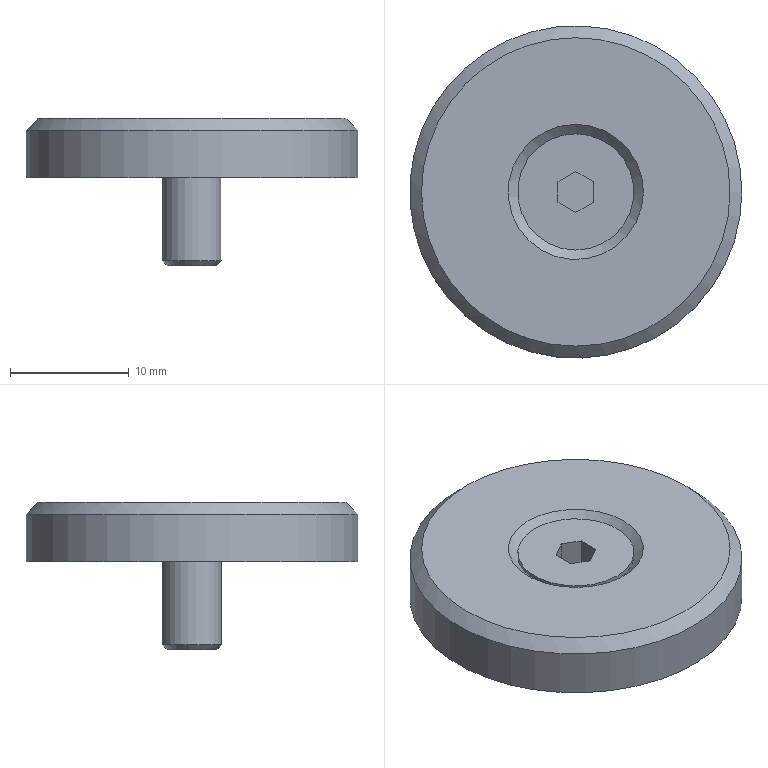Part | STEP file | STP | 2 solids | 19 faces | box 28 x 28 x 12.4 mm | volume 3112 mm3 | plane 11 | cylinder 4 | cone 4 | commonest cylinder face diameters 5 x1 5.5 x1 9.8 x1 28 x1
STEP:
#1=CARTESIAN_POINT('',(0.,0.,0.));
#2=DIRECTION('',(0.,0.,1.));
#3=DIRECTION('',(1.,0.,0.));
#4=AXIS2_PLACEMENT_3D('',#1,#2,#3);
#5=CARTESIAN_POINT('',(138.,294.1,-308.4));
#6=VERTEX_POINT('',#5);
#7=CARTESIAN_POINT('',(138.,289.9,-308.4));
#8=VERTEX_POINT('',#7);
#9=CARTESIAN_POINT('',(138.,292.,-308.4));
#10=DIRECTION('',(0.,0.,-1.));
#11=DIRECTION('',(0.,1.,0.));
#12=AXIS2_PLACEMENT_3D('',#9,#10,#11);
#13=CIRCLE('',#12,2.1);
#14=CARTESIAN_POINT('',(138.,292.,-308.4));
#15=DIRECTION('',(0.,0.,-1.));
#16=DIRECTION('',(0.,1.,0.));
#17=AXIS2_PLACEMENT_3D('',#14,#15,#16);
#18=PLANE('',#17);
#19=CARTESIAN_POINT('',(0.,0.));
#20=DIRECTION('',(1.,0.));
#21=AXIS2_PLACEMENT_2D('',#19,#20);
#22=CIRCLE('',#21,2.1);
#23=(GEOMETRIC_REPRESENTATION_CONTEXT(2)PARAMETRIC_REPRESENTATION_CONTEXT()REPRESENTATION_CONTEXT('',''));
#24=DEFINITIONAL_REPRESENTATION('',(#22),#23);
#25=PCURVE('',#18,#24);
#26=CARTESIAN_POINT('',(138.,292.,-308.));
#27=DIRECTION('',(0.,0.,1.));
#28=DIRECTION('',(0.,-1.,0.));
#29=AXIS2_PLACEMENT_3D('',#26,#27,#28);
#30=CONICAL_SURFACE('',#29,2.5,0.7854);
#31=CARTESIAN_POINT('',(3.142,-0.4));
#32=DIRECTION('',(-1.,0.));
#33=VECTOR('',#32,1.);
#34=LINE('',#31,#33);
#35=(GEOMETRIC_REPRESENTATION_CONTEXT(2)PARAMETRIC_REPRESENTATION_CONTEXT()REPRESENTATION_CONTEXT('',''));
#36=DEFINITIONAL_REPRESENTATION('',(#34),#35);
#37=PCURVE('',#30,#36);
#38=SURFACE_CURVE('',#13,(#25,#37),.PCURVE_S1.);
#39=EDGE_CURVE('',#6,#8,#38,.T.);
#40=ORIENTED_EDGE('',*,*,#39,.T.);
#41=CARTESIAN_POINT('',(138.,292.,-308.4));
#42=DIRECTION('',(0.,0.,-1.));
#43=DIRECTION('',(0.,1.,0.));
#44=AXIS2_PLACEMENT_3D('',#41,#42,#43);
#45=CIRCLE('',#44,2.1);
#46=CARTESIAN_POINT('',(0.,0.));
#47=DIRECTION('',(1.,0.));
#48=AXIS2_PLACEMENT_2D('',#46,#47);
#49=CIRCLE('',#48,2.1);
#50=(GEOMETRIC_REPRESENTATION_CONTEXT(2)PARAMETRIC_REPRESENTATION_CONTEXT()REPRESENTATION_CONTEXT('',''));
#51=DEFINITIONAL_REPRESENTATION('',(#49),#50);
#52=PCURVE('',#18,#51);
#53=CARTESIAN_POINT('',(9.425,-0.4));
#54=DIRECTION('',(-1.,0.));
#55=VECTOR('',#54,1.);
#56=LINE('',#53,#55);
#57=(GEOMETRIC_REPRESENTATION_CONTEXT(2)PARAMETRIC_REPRESENTATION_CONTEXT()REPRESENTATION_CONTEXT('',''));
#58=DEFINITIONAL_REPRESENTATION('',(#56),#57);
#59=PCURVE('',#30,#58);
#60=SURFACE_CURVE('',#45,(#52,#59),.PCURVE_S1.);
#61=EDGE_CURVE('',#8,#6,#60,.T.);
#62=ORIENTED_EDGE('',*,*,#61,.T.);
#63=EDGE_LOOP('',(#40,#62));
#64=FACE_BOUND('',#63,.T.);
#65=ADVANCED_FACE('',(#64),#18,.T.);
#66=CARTESIAN_POINT('',(138.,289.5,-308.));
#67=VERTEX_POINT('',#66);
#68=CARTESIAN_POINT('',(138.,292.,-308.));
#69=DIRECTION('',(0.,0.,1.));
#70=DIRECTION('',(0.,-1.,0.));
#71=AXIS2_PLACEMENT_3D('',#68,#69,#70);
#72=CIRCLE('',#71,2.5);
#73=CARTESIAN_POINT('',(138.,292.,-299.2));
#74=DIRECTION('',(0.,0.,-1.));
#75=DIRECTION('',(0.,1.,0.));
#76=AXIS2_PLACEMENT_3D('',#73,#74,#75);
#77=CYLINDRICAL_SURFACE('',#76,2.5);
#78=CARTESIAN_POINT('',(9.425,8.8));
#79=DIRECTION('',(-1.,0.));
#80=VECTOR('',#79,1.);
#81=LINE('',#78,#80);
#82=(GEOMETRIC_REPRESENTATION_CONTEXT(2)PARAMETRIC_REPRESENTATION_CONTEXT()REPRESENTATION_CONTEXT('',''));
#83=DEFINITIONAL_REPRESENTATION('',(#81),#82);
#84=PCURVE('',#77,#83);
#85=CARTESIAN_POINT('',(0.,0.));
#86=DIRECTION('',(1.,0.));
#87=VECTOR('',#86,1.);
#88=LINE('',#85,#87);
#89=(GEOMETRIC_REPRESENTATION_CONTEXT(2)PARAMETRIC_REPRESENTATION_CONTEXT()REPRESENTATION_CONTEXT('',''));
#90=DEFINITIONAL_REPRESENTATION('',(#88),#89);
#91=PCURVE('',#30,#90);
#92=SURFACE_CURVE('',#72,(#84,#91),.PCURVE_S1.);
#93=EDGE_CURVE('',#67,#67,#92,.T.);
#94=ORIENTED_EDGE('',*,*,#93,.T.);
#95=CARTESIAN_POINT('',(138.,289.5,-299.2));
#96=VERTEX_POINT('',#95);
#97=CARTESIAN_POINT('',(138.,289.5,-299.2));
#98=CARTESIAN_POINT('',(138.,289.5,-308.));
#99=B_SPLINE_CURVE_WITH_KNOTS('',1,(#97,#98),.UNSPECIFIED.,.F.,.F.,(2,2),(0.,8.8),.PIECEWISE_BEZIER_KNOTS.);
#100=CARTESIAN_POINT('',(3.142,0.));
#101=DIRECTION('',(0.,1.));
#102=VECTOR('',#101,1.);
#103=LINE('',#100,#102);
#104=(GEOMETRIC_REPRESENTATION_CONTEXT(2)PARAMETRIC_REPRESENTATION_CONTEXT()REPRESENTATION_CONTEXT('',''));
#105=DEFINITIONAL_REPRESENTATION('',(#103),#104);
#106=PCURVE('',#77,#105);
#107=CARTESIAN_POINT('',(9.425,0.));
#108=DIRECTION('',(0.,1.));
#109=VECTOR('',#108,1.);
#110=LINE('',#107,#109);
#111=(GEOMETRIC_REPRESENTATION_CONTEXT(2)PARAMETRIC_REPRESENTATION_CONTEXT()REPRESENTATION_CONTEXT('',''));
#112=DEFINITIONAL_REPRESENTATION('',(#110),#111);
#113=PCURVE('',#77,#112);
#114=SEAM_CURVE('',#99,(#106,#113),.PCURVE_S1.);
#115=EDGE_CURVE('',#96,#67,#114,.T.);
#116=ORIENTED_EDGE('',*,*,#115,.F.);
#117=CARTESIAN_POINT('',(138.,292.,-299.2));
#118=DIRECTION('',(0.,0.,1.));
#119=DIRECTION('',(0.,-1.,0.));
#120=AXIS2_PLACEMENT_3D('',#117,#118,#119);
#121=CIRCLE('',#120,2.5);
#122=CARTESIAN_POINT('',(9.425,0.));
#123=DIRECTION('',(-1.,0.));
#124=VECTOR('',#123,1.);
#125=LINE('',#122,#124);
#126=(GEOMETRIC_REPRESENTATION_CONTEXT(2)PARAMETRIC_REPRESENTATION_CONTEXT()REPRESENTATION_CONTEXT('',''));
#127=DEFINITIONAL_REPRESENTATION('',(#125),#126);
#128=PCURVE('',#77,#127);
#129=CARTESIAN_POINT('',(138.,292.,-299.2));
#130=DIRECTION('',(0.,0.,1.));
#131=DIRECTION('',(0.,1.,0.));
#132=AXIS2_PLACEMENT_3D('',#129,#130,#131);
#133=CONICAL_SURFACE('',#132,2.5,0.7854);
#134=CARTESIAN_POINT('',(3.142,0.));
#135=DIRECTION('',(1.,0.));
#136=VECTOR('',#135,1.);
#137=LINE('',#134,#136);
#138=(GEOMETRIC_REPRESENTATION_CONTEXT(2)PARAMETRIC_REPRESENTATION_CONTEXT()REPRESENTATION_CONTEXT('',''));
#139=DEFINITIONAL_REPRESENTATION('',(#137),#138);
#140=PCURVE('',#133,#139);
#141=SURFACE_CURVE('',#121,(#128,#140),.PCURVE_S1.);
#142=EDGE_CURVE('',#96,#96,#141,.T.);
#143=ORIENTED_EDGE('',*,*,#142,.F.);
#144=ORIENTED_EDGE('',*,*,#115,.T.);
#145=EDGE_LOOP('',(#94,#116,#143,#144));
#146=FACE_BOUND('',#145,.T.);
#147=ADVANCED_FACE('',(#146),#77,.T.);
#148=CARTESIAN_POINT('',(138.,287.1,-296.8));
#149=VERTEX_POINT('',#148);
#150=CARTESIAN_POINT('',(138.,292.,-296.8));
#151=DIRECTION('',(0.,0.,-1.));
#152=DIRECTION('',(0.,-1.,0.));
#153=AXIS2_PLACEMENT_3D('',#150,#151,#152);
#154=CIRCLE('',#153,4.9);
#155=CARTESIAN_POINT('',(9.425,2.4));
#156=DIRECTION('',(-1.,0.));
#157=VECTOR('',#156,1.);
#158=LINE('',#155,#157);
#159=(GEOMETRIC_REPRESENTATION_CONTEXT(2)PARAMETRIC_REPRESENTATION_CONTEXT()REPRESENTATION_CONTEXT('',''));
#160=DEFINITIONAL_REPRESENTATION('',(#158),#159);
#161=PCURVE('',#133,#160);
#162=CARTESIAN_POINT('',(138.,292.,-299.2));
#163=DIRECTION('',(0.,0.,1.));
#164=DIRECTION('',(0.,-1.,0.));
#165=AXIS2_PLACEMENT_3D('',#162,#163,#164);
#166=CYLINDRICAL_SURFACE('',#165,4.9);
#167=CARTESIAN_POINT('',(6.283,2.4));
#168=DIRECTION('',(-1.,0.));
#169=VECTOR('',#168,1.);
#170=LINE('',#167,#169);
#171=(GEOMETRIC_REPRESENTATION_CONTEXT(2)PARAMETRIC_REPRESENTATION_CONTEXT()REPRESENTATION_CONTEXT('',''));
#172=DEFINITIONAL_REPRESENTATION('',(#170),#171);
#173=PCURVE('',#166,#172);
#174=SURFACE_CURVE('',#154,(#161,#173),.PCURVE_S1.);
#175=EDGE_CURVE('',#149,#149,#174,.T.);
#176=ORIENTED_EDGE('',*,*,#175,.T.);
#177=CARTESIAN_POINT('',(138.,289.5,-299.2));
#178=CARTESIAN_POINT('',(138.,287.1,-296.8));
#179=B_SPLINE_CURVE_WITH_KNOTS('',1,(#177,#178),.UNSPECIFIED.,.F.,.F.,(2,2),(0.,3.394),.PIECEWISE_BEZIER_KNOTS.);
#180=CARTESIAN_POINT('',(3.142,0.));
#181=DIRECTION('',(0.,1.));
#182=VECTOR('',#181,1.);
#183=LINE('',#180,#182);
#184=(GEOMETRIC_REPRESENTATION_CONTEXT(2)PARAMETRIC_REPRESENTATION_CONTEXT()REPRESENTATION_CONTEXT('',''));
#185=DEFINITIONAL_REPRESENTATION('',(#183),#184);
#186=PCURVE('',#133,#185);
#187=CARTESIAN_POINT('',(9.425,0.));
#188=DIRECTION('',(0.,1.));
#189=VECTOR('',#188,1.);
#190=LINE('',#187,#189);
#191=(GEOMETRIC_REPRESENTATION_CONTEXT(2)PARAMETRIC_REPRESENTATION_CONTEXT()REPRESENTATION_CONTEXT('',''));
#192=DEFINITIONAL_REPRESENTATION('',(#190),#191);
#193=PCURVE('',#133,#192);
#194=SEAM_CURVE('',#179,(#186,#193),.PCURVE_S1.);
#195=EDGE_CURVE('',#96,#149,#194,.T.);
#196=ORIENTED_EDGE('',*,*,#195,.F.);
#197=ORIENTED_EDGE('',*,*,#142,.T.);
#198=ORIENTED_EDGE('',*,*,#195,.T.);
#199=EDGE_LOOP('',(#176,#196,#197,#198));
#200=FACE_BOUND('',#199,.T.);
#201=ADVANCED_FACE('',(#200),#133,.T.);
#202=CARTESIAN_POINT('',(138.,287.1,-296.4));
#203=VERTEX_POINT('',#202);
#204=CARTESIAN_POINT('',(138.,292.,-296.4));
#205=DIRECTION('',(0.,0.,1.));
#206=DIRECTION('',(0.,-1.,0.));
#207=AXIS2_PLACEMENT_3D('',#204,#205,#206);
#208=CIRCLE('',#207,4.9);
#209=CARTESIAN_POINT('',(0.,2.8));
#210=DIRECTION('',(1.,0.));
#211=VECTOR('',#210,1.);
#212=LINE('',#209,#211);
#213=(GEOMETRIC_REPRESENTATION_CONTEXT(2)PARAMETRIC_REPRESENTATION_CONTEXT()REPRESENTATION_CONTEXT('',''));
#214=DEFINITIONAL_REPRESENTATION('',(#212),#213);
#215=PCURVE('',#166,#214);
#216=CARTESIAN_POINT('',(138.,292.,-296.4));
#217=DIRECTION('',(0.,0.,1.));
#218=DIRECTION('',(0.,-1.,0.));
#219=AXIS2_PLACEMENT_3D('',#216,#217,#218);
#220=PLANE('',#219);
#221=CARTESIAN_POINT('',(0.,0.));
#222=DIRECTION('',(1.,0.));
#223=AXIS2_PLACEMENT_2D('',#221,#222);
#224=CIRCLE('',#223,4.9);
#225=(GEOMETRIC_REPRESENTATION_CONTEXT(2)PARAMETRIC_REPRESENTATION_CONTEXT()REPRESENTATION_CONTEXT('',''));
#226=DEFINITIONAL_REPRESENTATION('',(#224),#225);
#227=PCURVE('',#220,#226);
#228=SURFACE_CURVE('',#208,(#215,#227),.PCURVE_S1.);
#229=EDGE_CURVE('',#203,#203,#228,.T.);
#230=ORIENTED_EDGE('',*,*,#229,.F.);
#231=CARTESIAN_POINT('',(138.,287.1,-296.8));
#232=CARTESIAN_POINT('',(138.,287.1,-296.4));
#233=B_SPLINE_CURVE_WITH_KNOTS('',1,(#231,#232),.UNSPECIFIED.,.F.,.F.,(2,2),(2.4,2.8),.PIECEWISE_BEZIER_KNOTS.);
#234=CARTESIAN_POINT('',(0.,0.));
#235=DIRECTION('',(0.,1.));
#236=VECTOR('',#235,1.);
#237=LINE('',#234,#236);
#238=(GEOMETRIC_REPRESENTATION_CONTEXT(2)PARAMETRIC_REPRESENTATION_CONTEXT()REPRESENTATION_CONTEXT('',''));
#239=DEFINITIONAL_REPRESENTATION('',(#237),#238);
#240=PCURVE('',#166,#239);
#241=CARTESIAN_POINT('',(6.283,0.));
#242=DIRECTION('',(0.,1.));
#243=VECTOR('',#242,1.);
#244=LINE('',#241,#243);
#245=(GEOMETRIC_REPRESENTATION_CONTEXT(2)PARAMETRIC_REPRESENTATION_CONTEXT()REPRESENTATION_CONTEXT('',''));
#246=DEFINITIONAL_REPRESENTATION('',(#244),#245);
#247=PCURVE('',#166,#246);
#248=SEAM_CURVE('',#233,(#240,#247),.PCURVE_S1.);
#249=EDGE_CURVE('',#149,#203,#248,.T.);
#250=ORIENTED_EDGE('',*,*,#249,.F.);
#251=ORIENTED_EDGE('',*,*,#175,.F.);
#252=ORIENTED_EDGE('',*,*,#249,.T.);
#253=EDGE_LOOP('',(#230,#250,#251,#252));
#254=FACE_BOUND('',#253,.T.);
#255=ADVANCED_FACE('',(#254),#166,.T.);
#256=CARTESIAN_POINT('',(138.,290.268,-296.4));
#257=VERTEX_POINT('',#256);
#258=CARTESIAN_POINT('',(139.5,291.134,-296.4));
#259=VERTEX_POINT('',#258);
#260=CARTESIAN_POINT('',(138.,290.268,-296.4));
#261=DIRECTION('',(0.866,0.5,0.));
#262=VECTOR('',#261,1.);
#263=LINE('',#260,#262);
#264=CARTESIAN_POINT('',(1.732,0.));
#265=DIRECTION('',(-0.5,0.866));
#266=VECTOR('',#265,1.);
#267=LINE('',#264,#266);
#268=(GEOMETRIC_REPRESENTATION_CONTEXT(2)PARAMETRIC_REPRESENTATION_CONTEXT()REPRESENTATION_CONTEXT('',''));
#269=DEFINITIONAL_REPRESENTATION('',(#267),#268);
#270=PCURVE('',#220,#269);
#271=CARTESIAN_POINT('',(138.,290.268,-298.9));
#272=DIRECTION('',(0.5,-0.866,0.));
#273=DIRECTION('',(-0.866,-0.5,0.));
#274=AXIS2_PLACEMENT_3D('',#271,#272,#273);
#275=PLANE('',#274);
#276=CARTESIAN_POINT('',(0.,-2.5));
#277=DIRECTION('',(-1.,0.));
#278=VECTOR('',#277,1.);
#279=LINE('',#276,#278);
#280=(GEOMETRIC_REPRESENTATION_CONTEXT(2)PARAMETRIC_REPRESENTATION_CONTEXT()REPRESENTATION_CONTEXT('',''));
#281=DEFINITIONAL_REPRESENTATION('',(#279),#280);
#282=PCURVE('',#275,#281);
#283=SURFACE_CURVE('',#263,(#270,#282),.PCURVE_S1.);
#284=EDGE_CURVE('',#257,#259,#283,.T.);
#285=ORIENTED_EDGE('',*,*,#284,.F.);
#286=CARTESIAN_POINT('',(136.5,291.134,-296.4));
#287=VERTEX_POINT('',#286);
#288=CARTESIAN_POINT('',(136.5,291.134,-296.4));
#289=DIRECTION('',(0.866,-0.5,0.));
#290=VECTOR('',#289,1.);
#291=LINE('',#288,#290);
#292=CARTESIAN_POINT('',(0.866,-1.5));
#293=DIRECTION('',(0.5,0.866));
#294=VECTOR('',#293,1.);
#295=LINE('',#292,#294);
#296=(GEOMETRIC_REPRESENTATION_CONTEXT(2)PARAMETRIC_REPRESENTATION_CONTEXT()REPRESENTATION_CONTEXT('',''));
#297=DEFINITIONAL_REPRESENTATION('',(#295),#296);
#298=PCURVE('',#220,#297);
#299=CARTESIAN_POINT('',(136.5,291.134,-298.9));
#300=DIRECTION('',(-0.5,-0.866,0.));
#301=DIRECTION('',(-0.866,0.5,0.));
#302=AXIS2_PLACEMENT_3D('',#299,#300,#301);
#303=PLANE('',#302);
#304=CARTESIAN_POINT('',(0.,-2.5));
#305=DIRECTION('',(-1.,0.));
#306=VECTOR('',#305,1.);
#307=LINE('',#304,#306);
#308=(GEOMETRIC_REPRESENTATION_CONTEXT(2)PARAMETRIC_REPRESENTATION_CONTEXT()REPRESENTATION_CONTEXT('',''));
#309=DEFINITIONAL_REPRESENTATION('',(#307),#308);
#310=PCURVE('',#303,#309);
#311=SURFACE_CURVE('',#291,(#298,#310),.PCURVE_S1.);
#312=EDGE_CURVE('',#287,#257,#311,.T.);
#313=ORIENTED_EDGE('',*,*,#312,.F.);
#314=CARTESIAN_POINT('',(136.5,292.866,-296.4));
#315=VERTEX_POINT('',#314);
#316=CARTESIAN_POINT('',(136.5,292.866,-296.4));
#317=DIRECTION('',(0.,-1.,0.));
#318=VECTOR('',#317,1.);
#319=LINE('',#316,#318);
#320=CARTESIAN_POINT('',(-0.866,-1.5));
#321=DIRECTION('',(1.,0.));
#322=VECTOR('',#321,1.);
#323=LINE('',#320,#322);
#324=(GEOMETRIC_REPRESENTATION_CONTEXT(2)PARAMETRIC_REPRESENTATION_CONTEXT()REPRESENTATION_CONTEXT('',''));
#325=DEFINITIONAL_REPRESENTATION('',(#323),#324);
#326=PCURVE('',#220,#325);
#327=CARTESIAN_POINT('',(136.5,292.866,-298.9));
#328=DIRECTION('',(-1.,0.,0.));
#329=DIRECTION('',(0.,0.,1.));
#330=AXIS2_PLACEMENT_3D('',#327,#328,#329);
#331=PLANE('',#330);
#332=CARTESIAN_POINT('',(2.5,0.));
#333=DIRECTION('',(0.,-1.));
#334=VECTOR('',#333,1.);
#335=LINE('',#332,#334);
#336=(GEOMETRIC_REPRESENTATION_CONTEXT(2)PARAMETRIC_REPRESENTATION_CONTEXT()REPRESENTATION_CONTEXT('',''));
#337=DEFINITIONAL_REPRESENTATION('',(#335),#336);
#338=PCURVE('',#331,#337);
#339=SURFACE_CURVE('',#319,(#326,#338),.PCURVE_S1.);
#340=EDGE_CURVE('',#315,#287,#339,.T.);
#341=ORIENTED_EDGE('',*,*,#340,.F.);
#342=CARTESIAN_POINT('',(138.,293.732,-296.4));
#343=VERTEX_POINT('',#342);
#344=CARTESIAN_POINT('',(138.,293.732,-296.4));
#345=DIRECTION('',(-0.866,-0.5,0.));
#346=VECTOR('',#345,1.);
#347=LINE('',#344,#346);
#348=CARTESIAN_POINT('',(-1.732,0.));
#349=DIRECTION('',(0.5,-0.866));
#350=VECTOR('',#349,1.);
#351=LINE('',#348,#350);
#352=(GEOMETRIC_REPRESENTATION_CONTEXT(2)PARAMETRIC_REPRESENTATION_CONTEXT()REPRESENTATION_CONTEXT('',''));
#353=DEFINITIONAL_REPRESENTATION('',(#351),#352);
#354=PCURVE('',#220,#353);
#355=CARTESIAN_POINT('',(138.,293.732,-298.9));
#356=DIRECTION('',(-0.5,0.866,0.));
#357=DIRECTION('',(0.866,0.5,0.));
#358=AXIS2_PLACEMENT_3D('',#355,#356,#357);
#359=PLANE('',#358);
#360=CARTESIAN_POINT('',(0.,-2.5));
#361=DIRECTION('',(-1.,0.));
#362=VECTOR('',#361,1.);
#363=LINE('',#360,#362);
#364=(GEOMETRIC_REPRESENTATION_CONTEXT(2)PARAMETRIC_REPRESENTATION_CONTEXT()REPRESENTATION_CONTEXT('',''));
#365=DEFINITIONAL_REPRESENTATION('',(#363),#364);
#366=PCURVE('',#359,#365);
#367=SURFACE_CURVE('',#347,(#354,#366),.PCURVE_S1.);
#368=EDGE_CURVE('',#343,#315,#367,.T.);
#369=ORIENTED_EDGE('',*,*,#368,.F.);
#370=CARTESIAN_POINT('',(139.5,292.866,-296.4));
#371=VERTEX_POINT('',#370);
#372=CARTESIAN_POINT('',(139.5,292.866,-296.4));
#373=DIRECTION('',(-0.866,0.5,0.));
#374=VECTOR('',#373,1.);
#375=LINE('',#372,#374);
#376=CARTESIAN_POINT('',(-0.866,1.5));
#377=DIRECTION('',(-0.5,-0.866));
#378=VECTOR('',#377,1.);
#379=LINE('',#376,#378);
#380=(GEOMETRIC_REPRESENTATION_CONTEXT(2)PARAMETRIC_REPRESENTATION_CONTEXT()REPRESENTATION_CONTEXT('',''));
#381=DEFINITIONAL_REPRESENTATION('',(#379),#380);
#382=PCURVE('',#220,#381);
#383=CARTESIAN_POINT('',(139.5,292.866,-298.9));
#384=DIRECTION('',(0.5,0.866,0.));
#385=DIRECTION('',(0.866,-0.5,0.));
#386=AXIS2_PLACEMENT_3D('',#383,#384,#385);
#387=PLANE('',#386);
#388=CARTESIAN_POINT('',(0.,-2.5));
#389=DIRECTION('',(-1.,0.));
#390=VECTOR('',#389,1.);
#391=LINE('',#388,#390);
#392=(GEOMETRIC_REPRESENTATION_CONTEXT(2)PARAMETRIC_REPRESENTATION_CONTEXT()REPRESENTATION_CONTEXT('',''));
#393=DEFINITIONAL_REPRESENTATION('',(#391),#392);
#394=PCURVE('',#387,#393);
#395=SURFACE_CURVE('',#375,(#382,#394),.PCURVE_S1.);
#396=EDGE_CURVE('',#371,#343,#395,.T.);
#397=ORIENTED_EDGE('',*,*,#396,.F.);
#398=CARTESIAN_POINT('',(139.5,291.134,-296.4));
#399=DIRECTION('',(0.,1.,0.));
#400=VECTOR('',#399,1.);
#401=LINE('',#398,#400);
#402=CARTESIAN_POINT('',(0.866,1.5));
#403=DIRECTION('',(-1.,0.));
#404=VECTOR('',#403,1.);
#405=LINE('',#402,#404);
#406=(GEOMETRIC_REPRESENTATION_CONTEXT(2)PARAMETRIC_REPRESENTATION_CONTEXT()REPRESENTATION_CONTEXT('',''));
#407=DEFINITIONAL_REPRESENTATION('',(#405),#406);
#408=PCURVE('',#220,#407);
#409=CARTESIAN_POINT('',(139.5,291.134,-298.9));
#410=DIRECTION('',(1.,0.,0.));
#411=DIRECTION('',(0.,0.,-1.));
#412=AXIS2_PLACEMENT_3D('',#409,#410,#411);
#413=PLANE('',#412);
#414=CARTESIAN_POINT('',(-2.5,0.));
#415=DIRECTION('',(0.,1.));
#416=VECTOR('',#415,1.);
#417=LINE('',#414,#416);
#418=(GEOMETRIC_REPRESENTATION_CONTEXT(2)PARAMETRIC_REPRESENTATION_CONTEXT()REPRESENTATION_CONTEXT('',''));
#419=DEFINITIONAL_REPRESENTATION('',(#417),#418);
#420=PCURVE('',#413,#419);
#421=SURFACE_CURVE('',#401,(#408,#420),.PCURVE_S1.);
#422=EDGE_CURVE('',#259,#371,#421,.T.);
#423=ORIENTED_EDGE('',*,*,#422,.F.);
#424=EDGE_LOOP('',(#285,#313,#341,#369,#397,#423));
#425=FACE_BOUND('',#424,.T.);
#426=ORIENTED_EDGE('',*,*,#229,.T.);
#427=EDGE_LOOP('',(#426));
#428=FACE_BOUND('',#427,.T.);
#429=ADVANCED_FACE('',(#425,#428),#220,.T.);
#430=ORIENTED_EDGE('',*,*,#284,.T.);
#431=CARTESIAN_POINT('',(139.5,291.134,-298.9));
#432=VERTEX_POINT('',#431);
#433=CARTESIAN_POINT('',(139.5,291.134,-298.9));
#434=DIRECTION('',(0.,0.,1.));
#435=VECTOR('',#434,1.);
#436=LINE('',#433,#435);
#437=CARTESIAN_POINT('',(-1.732,0.));
#438=DIRECTION('',(0.,-1.));
#439=VECTOR('',#438,1.);
#440=LINE('',#437,#439);
#441=(GEOMETRIC_REPRESENTATION_CONTEXT(2)PARAMETRIC_REPRESENTATION_CONTEXT()REPRESENTATION_CONTEXT('',''));
#442=DEFINITIONAL_REPRESENTATION('',(#440),#441);
#443=PCURVE('',#275,#442);
#444=CARTESIAN_POINT('',(0.,0.));
#445=DIRECTION('',(-1.,0.));
#446=VECTOR('',#445,1.);
#447=LINE('',#444,#446);
#448=(GEOMETRIC_REPRESENTATION_CONTEXT(2)PARAMETRIC_REPRESENTATION_CONTEXT()REPRESENTATION_CONTEXT('',''));
#449=DEFINITIONAL_REPRESENTATION('',(#447),#448);
#450=PCURVE('',#413,#449);
#451=SURFACE_CURVE('',#436,(#443,#450),.PCURVE_S1.);
#452=EDGE_CURVE('',#432,#259,#451,.T.);
#453=ORIENTED_EDGE('',*,*,#452,.F.);
#454=CARTESIAN_POINT('',(138.,290.268,-298.9));
#455=VERTEX_POINT('',#454);
#456=CARTESIAN_POINT('',(138.,290.268,-298.9));
#457=DIRECTION('',(0.866,0.5,0.));
#458=VECTOR('',#457,1.);
#459=LINE('',#456,#458);
#460=CARTESIAN_POINT('',(0.,0.));
#461=DIRECTION('',(-1.,0.));
#462=VECTOR('',#461,1.);
#463=LINE('',#460,#462);
#464=(GEOMETRIC_REPRESENTATION_CONTEXT(2)PARAMETRIC_REPRESENTATION_CONTEXT()REPRESENTATION_CONTEXT('',''));
#465=DEFINITIONAL_REPRESENTATION('',(#463),#464);
#466=PCURVE('',#275,#465);
#467=CARTESIAN_POINT('',(141.,292.,-298.9));
#468=DIRECTION('',(0.,0.,1.));
#469=DIRECTION('',(0.,-1.,0.));
#470=AXIS2_PLACEMENT_3D('',#467,#468,#469);
#471=PLANE('',#470);
#472=CARTESIAN_POINT('',(1.732,-3.));
#473=DIRECTION('',(-0.5,0.866));
#474=VECTOR('',#473,1.);
#475=LINE('',#472,#474);
#476=(GEOMETRIC_REPRESENTATION_CONTEXT(2)PARAMETRIC_REPRESENTATION_CONTEXT()REPRESENTATION_CONTEXT('',''));
#477=DEFINITIONAL_REPRESENTATION('',(#475),#476);
#478=PCURVE('',#471,#477);
#479=SURFACE_CURVE('',#459,(#466,#478),.PCURVE_S1.);
#480=EDGE_CURVE('',#455,#432,#479,.T.);
#481=ORIENTED_EDGE('',*,*,#480,.F.);
#482=CARTESIAN_POINT('',(138.,290.268,-298.9));
#483=DIRECTION('',(0.,0.,1.));
#484=VECTOR('',#483,1.);
#485=LINE('',#482,#484);
#486=CARTESIAN_POINT('',(0.,0.));
#487=DIRECTION('',(0.,-1.));
#488=VECTOR('',#487,1.);
#489=LINE('',#486,#488);
#490=(GEOMETRIC_REPRESENTATION_CONTEXT(2)PARAMETRIC_REPRESENTATION_CONTEXT()REPRESENTATION_CONTEXT('',''));
#491=DEFINITIONAL_REPRESENTATION('',(#489),#490);
#492=PCURVE('',#275,#491);
#493=CARTESIAN_POINT('',(-1.732,0.));
#494=DIRECTION('',(0.,-1.));
#495=VECTOR('',#494,1.);
#496=LINE('',#493,#495);
#497=(GEOMETRIC_REPRESENTATION_CONTEXT(2)PARAMETRIC_REPRESENTATION_CONTEXT()REPRESENTATION_CONTEXT('',''));
#498=DEFINITIONAL_REPRESENTATION('',(#496),#497);
#499=PCURVE('',#303,#498);
#500=SURFACE_CURVE('',#485,(#492,#499),.PCURVE_S1.);
#501=EDGE_CURVE('',#455,#257,#500,.T.);
#502=ORIENTED_EDGE('',*,*,#501,.T.);
#503=EDGE_LOOP('',(#430,#453,#481,#502));
#504=FACE_BOUND('',#503,.T.);
#505=ADVANCED_FACE('',(#504),#275,.F.);
#506=ORIENTED_EDGE('',*,*,#422,.T.);
#507=CARTESIAN_POINT('',(139.5,292.866,-298.9));
#508=VERTEX_POINT('',#507);
#509=CARTESIAN_POINT('',(139.5,292.866,-298.9));
#510=DIRECTION('',(0.,0.,1.));
#511=VECTOR('',#510,1.);
#512=LINE('',#509,#511);
#513=CARTESIAN_POINT('',(0.,1.732));
#514=DIRECTION('',(-1.,0.));
#515=VECTOR('',#514,1.);
#516=LINE('',#513,#515);
#517=(GEOMETRIC_REPRESENTATION_CONTEXT(2)PARAMETRIC_REPRESENTATION_CONTEXT()REPRESENTATION_CONTEXT('',''));
#518=DEFINITIONAL_REPRESENTATION('',(#516),#517);
#519=PCURVE('',#413,#518);
#520=CARTESIAN_POINT('',(0.,0.));
#521=DIRECTION('',(0.,-1.));
#522=VECTOR('',#521,1.);
#523=LINE('',#520,#522);
#524=(GEOMETRIC_REPRESENTATION_CONTEXT(2)PARAMETRIC_REPRESENTATION_CONTEXT()REPRESENTATION_CONTEXT('',''));
#525=DEFINITIONAL_REPRESENTATION('',(#523),#524);
#526=PCURVE('',#387,#525);
#527=SURFACE_CURVE('',#512,(#519,#526),.PCURVE_S1.);
#528=EDGE_CURVE('',#508,#371,#527,.T.);
#529=ORIENTED_EDGE('',*,*,#528,.F.);
#530=CARTESIAN_POINT('',(139.5,291.134,-298.9));
#531=DIRECTION('',(0.,1.,0.));
#532=VECTOR('',#531,1.);
#533=LINE('',#530,#532);
#534=CARTESIAN_POINT('',(0.,0.));
#535=DIRECTION('',(0.,1.));
#536=VECTOR('',#535,1.);
#537=LINE('',#534,#536);
#538=(GEOMETRIC_REPRESENTATION_CONTEXT(2)PARAMETRIC_REPRESENTATION_CONTEXT()REPRESENTATION_CONTEXT('',''));
#539=DEFINITIONAL_REPRESENTATION('',(#537),#538);
#540=PCURVE('',#413,#539);
#541=CARTESIAN_POINT('',(0.866,-1.5));
#542=DIRECTION('',(-1.,0.));
#543=VECTOR('',#542,1.);
#544=LINE('',#541,#543);
#545=(GEOMETRIC_REPRESENTATION_CONTEXT(2)PARAMETRIC_REPRESENTATION_CONTEXT()REPRESENTATION_CONTEXT('',''));
#546=DEFINITIONAL_REPRESENTATION('',(#544),#545);
#547=PCURVE('',#471,#546);
#548=SURFACE_CURVE('',#533,(#540,#547),.PCURVE_S1.);
#549=EDGE_CURVE('',#432,#508,#548,.T.);
#550=ORIENTED_EDGE('',*,*,#549,.F.);
#551=ORIENTED_EDGE('',*,*,#452,.T.);
#552=EDGE_LOOP('',(#506,#529,#550,#551));
#553=FACE_BOUND('',#552,.T.);
#554=ADVANCED_FACE('',(#553),#413,.F.);
#555=ORIENTED_EDGE('',*,*,#396,.T.);
#556=CARTESIAN_POINT('',(138.,293.732,-298.9));
#557=VERTEX_POINT('',#556);
#558=CARTESIAN_POINT('',(138.,293.732,-298.9));
#559=DIRECTION('',(0.,0.,1.));
#560=VECTOR('',#559,1.);
#561=LINE('',#558,#560);
#562=CARTESIAN_POINT('',(-1.732,0.));
#563=DIRECTION('',(0.,-1.));
#564=VECTOR('',#563,1.);
#565=LINE('',#562,#564);
#566=(GEOMETRIC_REPRESENTATION_CONTEXT(2)PARAMETRIC_REPRESENTATION_CONTEXT()REPRESENTATION_CONTEXT('',''));
#567=DEFINITIONAL_REPRESENTATION('',(#565),#566);
#568=PCURVE('',#387,#567);
#569=CARTESIAN_POINT('',(0.,0.));
#570=DIRECTION('',(0.,-1.));
#571=VECTOR('',#570,1.);
#572=LINE('',#569,#571);
#573=(GEOMETRIC_REPRESENTATION_CONTEXT(2)PARAMETRIC_REPRESENTATION_CONTEXT()REPRESENTATION_CONTEXT('',''));
#574=DEFINITIONAL_REPRESENTATION('',(#572),#573);
#575=PCURVE('',#359,#574);
#576=SURFACE_CURVE('',#561,(#568,#575),.PCURVE_S1.);
#577=EDGE_CURVE('',#557,#343,#576,.T.);
#578=ORIENTED_EDGE('',*,*,#577,.F.);
#579=CARTESIAN_POINT('',(139.5,292.866,-298.9));
#580=DIRECTION('',(-0.866,0.5,0.));
#581=VECTOR('',#580,1.);
#582=LINE('',#579,#581);
#583=CARTESIAN_POINT('',(0.,0.));
#584=DIRECTION('',(-1.,0.));
#585=VECTOR('',#584,1.);
#586=LINE('',#583,#585);
#587=(GEOMETRIC_REPRESENTATION_CONTEXT(2)PARAMETRIC_REPRESENTATION_CONTEXT()REPRESENTATION_CONTEXT('',''));
#588=DEFINITIONAL_REPRESENTATION('',(#586),#587);
#589=PCURVE('',#387,#588);
#590=CARTESIAN_POINT('',(-0.866,-1.5));
#591=DIRECTION('',(-0.5,-0.866));
#592=VECTOR('',#591,1.);
#593=LINE('',#590,#592);
#594=(GEOMETRIC_REPRESENTATION_CONTEXT(2)PARAMETRIC_REPRESENTATION_CONTEXT()REPRESENTATION_CONTEXT('',''));
#595=DEFINITIONAL_REPRESENTATION('',(#593),#594);
#596=PCURVE('',#471,#595);
#597=SURFACE_CURVE('',#582,(#589,#596),.PCURVE_S1.);
#598=EDGE_CURVE('',#508,#557,#597,.T.);
#599=ORIENTED_EDGE('',*,*,#598,.F.);
#600=ORIENTED_EDGE('',*,*,#528,.T.);
#601=EDGE_LOOP('',(#555,#578,#599,#600));
#602=FACE_BOUND('',#601,.T.);
#603=ADVANCED_FACE('',(#602),#387,.F.);
#604=ORIENTED_EDGE('',*,*,#368,.T.);
#605=CARTESIAN_POINT('',(136.5,292.866,-298.9));
#606=VERTEX_POINT('',#605);
#607=CARTESIAN_POINT('',(136.5,292.866,-298.9));
#608=DIRECTION('',(0.,0.,1.));
#609=VECTOR('',#608,1.);
#610=LINE('',#607,#609);
#611=CARTESIAN_POINT('',(-1.732,0.));
#612=DIRECTION('',(0.,-1.));
#613=VECTOR('',#612,1.);
#614=LINE('',#611,#613);
#615=(GEOMETRIC_REPRESENTATION_CONTEXT(2)PARAMETRIC_REPRESENTATION_CONTEXT()REPRESENTATION_CONTEXT('',''));
#616=DEFINITIONAL_REPRESENTATION('',(#614),#615);
#617=PCURVE('',#359,#616);
#618=CARTESIAN_POINT('',(0.,0.));
#619=DIRECTION('',(1.,0.));
#620=VECTOR('',#619,1.);
#621=LINE('',#618,#620);
#622=(GEOMETRIC_REPRESENTATION_CONTEXT(2)PARAMETRIC_REPRESENTATION_CONTEXT()REPRESENTATION_CONTEXT('',''));
#623=DEFINITIONAL_REPRESENTATION('',(#621),#622);
#624=PCURVE('',#331,#623);
#625=SURFACE_CURVE('',#610,(#617,#624),.PCURVE_S1.);
#626=EDGE_CURVE('',#606,#315,#625,.T.);
#627=ORIENTED_EDGE('',*,*,#626,.F.);
#628=CARTESIAN_POINT('',(138.,293.732,-298.9));
#629=DIRECTION('',(-0.866,-0.5,0.));
#630=VECTOR('',#629,1.);
#631=LINE('',#628,#630);
#632=CARTESIAN_POINT('',(0.,0.));
#633=DIRECTION('',(-1.,0.));
#634=VECTOR('',#633,1.);
#635=LINE('',#632,#634);
#636=(GEOMETRIC_REPRESENTATION_CONTEXT(2)PARAMETRIC_REPRESENTATION_CONTEXT()REPRESENTATION_CONTEXT('',''));
#637=DEFINITIONAL_REPRESENTATION('',(#635),#636);
#638=PCURVE('',#359,#637);
#639=CARTESIAN_POINT('',(-1.732,-3.));
#640=DIRECTION('',(0.5,-0.866));
#641=VECTOR('',#640,1.);
#642=LINE('',#639,#641);
#643=(GEOMETRIC_REPRESENTATION_CONTEXT(2)PARAMETRIC_REPRESENTATION_CONTEXT()REPRESENTATION_CONTEXT('',''));
#644=DEFINITIONAL_REPRESENTATION('',(#642),#643);
#645=PCURVE('',#471,#644);
#646=SURFACE_CURVE('',#631,(#638,#645),.PCURVE_S1.);
#647=EDGE_CURVE('',#557,#606,#646,.T.);
#648=ORIENTED_EDGE('',*,*,#647,.F.);
#649=ORIENTED_EDGE('',*,*,#577,.T.);
#650=EDGE_LOOP('',(#604,#627,#648,#649));
#651=FACE_BOUND('',#650,.T.);
#652=ADVANCED_FACE('',(#651),#359,.F.);
#653=ORIENTED_EDGE('',*,*,#340,.T.);
#654=CARTESIAN_POINT('',(136.5,291.134,-298.9));
#655=VERTEX_POINT('',#654);
#656=CARTESIAN_POINT('',(136.5,291.134,-298.9));
#657=DIRECTION('',(0.,0.,1.));
#658=VECTOR('',#657,1.);
#659=LINE('',#656,#658);
#660=CARTESIAN_POINT('',(0.,-1.732));
#661=DIRECTION('',(1.,0.));
#662=VECTOR('',#661,1.);
#663=LINE('',#660,#662);
#664=(GEOMETRIC_REPRESENTATION_CONTEXT(2)PARAMETRIC_REPRESENTATION_CONTEXT()REPRESENTATION_CONTEXT('',''));
#665=DEFINITIONAL_REPRESENTATION('',(#663),#664);
#666=PCURVE('',#331,#665);
#667=CARTESIAN_POINT('',(0.,0.));
#668=DIRECTION('',(0.,-1.));
#669=VECTOR('',#668,1.);
#670=LINE('',#667,#669);
#671=(GEOMETRIC_REPRESENTATION_CONTEXT(2)PARAMETRIC_REPRESENTATION_CONTEXT()REPRESENTATION_CONTEXT('',''));
#672=DEFINITIONAL_REPRESENTATION('',(#670),#671);
#673=PCURVE('',#303,#672);
#674=SURFACE_CURVE('',#659,(#666,#673),.PCURVE_S1.);
#675=EDGE_CURVE('',#655,#287,#674,.T.);
#676=ORIENTED_EDGE('',*,*,#675,.F.);
#677=CARTESIAN_POINT('',(136.5,292.866,-298.9));
#678=DIRECTION('',(0.,-1.,0.));
#679=VECTOR('',#678,1.);
#680=LINE('',#677,#679);
#681=CARTESIAN_POINT('',(0.,0.));
#682=DIRECTION('',(0.,-1.));
#683=VECTOR('',#682,1.);
#684=LINE('',#681,#683);
#685=(GEOMETRIC_REPRESENTATION_CONTEXT(2)PARAMETRIC_REPRESENTATION_CONTEXT()REPRESENTATION_CONTEXT('',''));
#686=DEFINITIONAL_REPRESENTATION('',(#684),#685);
#687=PCURVE('',#331,#686);
#688=CARTESIAN_POINT('',(-0.866,-4.5));
#689=DIRECTION('',(1.,0.));
#690=VECTOR('',#689,1.);
#691=LINE('',#688,#690);
#692=(GEOMETRIC_REPRESENTATION_CONTEXT(2)PARAMETRIC_REPRESENTATION_CONTEXT()REPRESENTATION_CONTEXT('',''));
#693=DEFINITIONAL_REPRESENTATION('',(#691),#692);
#694=PCURVE('',#471,#693);
#695=SURFACE_CURVE('',#680,(#687,#694),.PCURVE_S1.);
#696=EDGE_CURVE('',#606,#655,#695,.T.);
#697=ORIENTED_EDGE('',*,*,#696,.F.);
#698=ORIENTED_EDGE('',*,*,#626,.T.);
#699=EDGE_LOOP('',(#653,#676,#697,#698));
#700=FACE_BOUND('',#699,.T.);
#701=ADVANCED_FACE('',(#700),#331,.F.);
#702=ORIENTED_EDGE('',*,*,#312,.T.);
#703=ORIENTED_EDGE('',*,*,#501,.F.);
#704=CARTESIAN_POINT('',(136.5,291.134,-298.9));
#705=DIRECTION('',(0.866,-0.5,0.));
#706=VECTOR('',#705,1.);
#707=LINE('',#704,#706);
#708=CARTESIAN_POINT('',(0.,0.));
#709=DIRECTION('',(-1.,0.));
#710=VECTOR('',#709,1.);
#711=LINE('',#708,#710);
#712=(GEOMETRIC_REPRESENTATION_CONTEXT(2)PARAMETRIC_REPRESENTATION_CONTEXT()REPRESENTATION_CONTEXT('',''));
#713=DEFINITIONAL_REPRESENTATION('',(#711),#712);
#714=PCURVE('',#303,#713);
#715=CARTESIAN_POINT('',(0.866,-4.5));
#716=DIRECTION('',(0.5,0.866));
#717=VECTOR('',#716,1.);
#718=LINE('',#715,#717);
#719=(GEOMETRIC_REPRESENTATION_CONTEXT(2)PARAMETRIC_REPRESENTATION_CONTEXT()REPRESENTATION_CONTEXT('',''));
#720=DEFINITIONAL_REPRESENTATION('',(#718),#719);
#721=PCURVE('',#471,#720);
#722=SURFACE_CURVE('',#707,(#714,#721),.PCURVE_S1.);
#723=EDGE_CURVE('',#655,#455,#722,.T.);
#724=ORIENTED_EDGE('',*,*,#723,.F.);
#725=ORIENTED_EDGE('',*,*,#675,.T.);
#726=EDGE_LOOP('',(#702,#703,#724,#725));
#727=FACE_BOUND('',#726,.T.);
#728=ADVANCED_FACE('',(#727),#303,.F.);
#729=ORIENTED_EDGE('',*,*,#480,.T.);
#730=ORIENTED_EDGE('',*,*,#549,.T.);
#731=ORIENTED_EDGE('',*,*,#598,.T.);
#732=ORIENTED_EDGE('',*,*,#647,.T.);
#733=ORIENTED_EDGE('',*,*,#696,.T.);
#734=ORIENTED_EDGE('',*,*,#723,.T.);
#735=EDGE_LOOP('',(#729,#730,#731,#732,#733,#734));
#736=FACE_BOUND('',#735,.T.);
#737=ADVANCED_FACE('',(#736),#471,.T.);
#738=ORIENTED_EDGE('',*,*,#61,.F.);
#739=CARTESIAN_POINT('',(138.,289.9,-308.4));
#740=CARTESIAN_POINT('',(138.,289.5,-308.));
#741=B_SPLINE_CURVE_WITH_KNOTS('',1,(#739,#740),.UNSPECIFIED.,.F.,.F.,(2,2),(-0.5657,0.),.PIECEWISE_BEZIER_KNOTS.);
#742=CARTESIAN_POINT('',(6.283,0.));
#743=DIRECTION('',(0.,1.));
#744=VECTOR('',#743,1.);
#745=LINE('',#742,#744);
#746=(GEOMETRIC_REPRESENTATION_CONTEXT(2)PARAMETRIC_REPRESENTATION_CONTEXT()REPRESENTATION_CONTEXT('',''));
#747=DEFINITIONAL_REPRESENTATION('',(#745),#746);
#748=PCURVE('',#30,#747);
#749=CARTESIAN_POINT('',(0.,0.));
#750=DIRECTION('',(0.,1.));
#751=VECTOR('',#750,1.);
#752=LINE('',#749,#751);
#753=(GEOMETRIC_REPRESENTATION_CONTEXT(2)PARAMETRIC_REPRESENTATION_CONTEXT()REPRESENTATION_CONTEXT('',''));
#754=DEFINITIONAL_REPRESENTATION('',(#752),#753);
#755=PCURVE('',#30,#754);
#756=SEAM_CURVE('',#741,(#748,#755),.PCURVE_S1.);
#757=EDGE_CURVE('',#8,#67,#756,.T.);
#758=ORIENTED_EDGE('',*,*,#757,.T.);
#759=ORIENTED_EDGE('',*,*,#93,.F.);
#760=ORIENTED_EDGE('',*,*,#757,.F.);
#761=ORIENTED_EDGE('',*,*,#39,.F.);
#762=EDGE_LOOP('',(#738,#758,#759,#760,#761));
#763=FACE_BOUND('',#762,.T.);
#764=ADVANCED_FACE('',(#763),#30,.T.);
#765=CLOSED_SHELL('',(#65,#147,#201,#255,#429,#505,#554,#603,#652,#701,#728,#737,#764));
#766=MANIFOLD_SOLID_BREP('',#765);
#767=CARTESIAN_POINT('',(152.,292.,-297.));
#768=VERTEX_POINT('',#767);
#769=CARTESIAN_POINT('',(138.,292.,-297.));
#770=DIRECTION('',(0.,0.,-1.));
#771=DIRECTION('',(1.,0.,0.));
#772=AXIS2_PLACEMENT_3D('',#769,#770,#771);
#773=CIRCLE('',#772,14.);
#774=CARTESIAN_POINT('',(138.,292.,-301.));
#775=DIRECTION('',(0.,0.,1.));
#776=DIRECTION('',(1.,0.,0.));
#777=AXIS2_PLACEMENT_3D('',#774,#775,#776);
#778=CYLINDRICAL_SURFACE('',#777,14.);
#779=CARTESIAN_POINT('',(6.283,4.));
#780=DIRECTION('',(-1.,0.));
#781=VECTOR('',#780,1.);
#782=LINE('',#779,#781);
#783=(GEOMETRIC_REPRESENTATION_CONTEXT(2)PARAMETRIC_REPRESENTATION_CONTEXT()REPRESENTATION_CONTEXT('',''));
#784=DEFINITIONAL_REPRESENTATION('',(#782),#783);
#785=PCURVE('',#778,#784);
#786=CARTESIAN_POINT('',(138.,292.,-296.));
#787=DIRECTION('',(0.,0.,-1.));
#788=DIRECTION('',(-1.,0.,0.));
#789=AXIS2_PLACEMENT_3D('',#786,#787,#788);
#790=CONICAL_SURFACE('',#789,13.,0.7854);
#791=CARTESIAN_POINT('',(3.142,1.));
#792=DIRECTION('',(1.,0.));
#793=VECTOR('',#792,1.);
#794=LINE('',#791,#793);
#795=(GEOMETRIC_REPRESENTATION_CONTEXT(2)PARAMETRIC_REPRESENTATION_CONTEXT()REPRESENTATION_CONTEXT('',''));
#796=DEFINITIONAL_REPRESENTATION('',(#794),#795);
#797=PCURVE('',#790,#796);
#798=SURFACE_CURVE('',#773,(#785,#797),.PCURVE_S1.);
#799=EDGE_CURVE('',#768,#768,#798,.T.);
#800=ORIENTED_EDGE('',*,*,#799,.T.);
#801=CARTESIAN_POINT('',(152.,292.,-301.));
#802=VERTEX_POINT('',#801);
#803=CARTESIAN_POINT('',(152.,292.,-301.));
#804=CARTESIAN_POINT('',(152.,292.,-297.));
#805=B_SPLINE_CURVE_WITH_KNOTS('',1,(#803,#804),.UNSPECIFIED.,.F.,.F.,(2,2),(0.,4.),.PIECEWISE_BEZIER_KNOTS.);
#806=CARTESIAN_POINT('',(0.,0.));
#807=DIRECTION('',(0.,1.));
#808=VECTOR('',#807,1.);
#809=LINE('',#806,#808);
#810=(GEOMETRIC_REPRESENTATION_CONTEXT(2)PARAMETRIC_REPRESENTATION_CONTEXT()REPRESENTATION_CONTEXT('',''));
#811=DEFINITIONAL_REPRESENTATION('',(#809),#810);
#812=PCURVE('',#778,#811);
#813=CARTESIAN_POINT('',(6.283,0.));
#814=DIRECTION('',(0.,1.));
#815=VECTOR('',#814,1.);
#816=LINE('',#813,#815);
#817=(GEOMETRIC_REPRESENTATION_CONTEXT(2)PARAMETRIC_REPRESENTATION_CONTEXT()REPRESENTATION_CONTEXT('',''));
#818=DEFINITIONAL_REPRESENTATION('',(#816),#817);
#819=PCURVE('',#778,#818);
#820=SEAM_CURVE('',#805,(#812,#819),.PCURVE_S1.);
#821=EDGE_CURVE('',#802,#768,#820,.T.);
#822=ORIENTED_EDGE('',*,*,#821,.F.);
#823=CARTESIAN_POINT('',(138.,292.,-301.));
#824=DIRECTION('',(0.,0.,-1.));
#825=DIRECTION('',(1.,0.,0.));
#826=AXIS2_PLACEMENT_3D('',#823,#824,#825);
#827=CIRCLE('',#826,14.);
#828=CARTESIAN_POINT('',(6.283,0.));
#829=DIRECTION('',(-1.,0.));
#830=VECTOR('',#829,1.);
#831=LINE('',#828,#830);
#832=(GEOMETRIC_REPRESENTATION_CONTEXT(2)PARAMETRIC_REPRESENTATION_CONTEXT()REPRESENTATION_CONTEXT('',''));
#833=DEFINITIONAL_REPRESENTATION('',(#831),#832);
#834=PCURVE('',#778,#833);
#835=CARTESIAN_POINT('',(138.,292.,-301.));
#836=DIRECTION('',(0.,0.,1.));
#837=DIRECTION('',(1.,0.,0.));
#838=AXIS2_PLACEMENT_3D('',#835,#836,#837);
#839=PLANE('',#838);
#840=CARTESIAN_POINT('',(14.,0.));
#841=CARTESIAN_POINT('',(14.,-24.249));
#842=CARTESIAN_POINT('',(-7.,-12.124));
#843=CARTESIAN_POINT('',(-28.,0.));
#844=CARTESIAN_POINT('',(-7.,12.124));
#845=CARTESIAN_POINT('',(14.,24.249));
#846=CARTESIAN_POINT('',(14.,0.));
#847=(BOUNDED_CURVE()B_SPLINE_CURVE(2,(#840,#841,#842,#843,#844,#845,#846),.UNSPECIFIED.,.T.,.F.)B_SPLINE_CURVE_WITH_KNOTS((1,2,2,2,2,1),(-2.094,0.,2.094,4.189,6.283,8.378),.UNSPECIFIED.)CURVE()GEOMETRIC_REPRESENTATION_ITEM()RATIONAL_B_SPLINE_CURVE((1.,0.5,1.,0.5,1.,0.5,1.))REPRESENTATION_ITEM(''));
#848=(GEOMETRIC_REPRESENTATION_CONTEXT(2)PARAMETRIC_REPRESENTATION_CONTEXT()REPRESENTATION_CONTEXT('',''));
#849=DEFINITIONAL_REPRESENTATION('',(#847),#848);
#850=PCURVE('',#839,#849);
#851=SURFACE_CURVE('',#827,(#834,#850),.PCURVE_S1.);
#852=EDGE_CURVE('',#802,#802,#851,.T.);
#853=ORIENTED_EDGE('',*,*,#852,.F.);
#854=ORIENTED_EDGE('',*,*,#821,.T.);
#855=EDGE_LOOP('',(#800,#822,#853,#854));
#856=FACE_BOUND('',#855,.T.);
#857=ADVANCED_FACE('',(#856),#778,.T.);
#858=ORIENTED_EDGE('',*,*,#852,.T.);
#859=EDGE_LOOP('',(#858));
#860=FACE_BOUND('',#859,.T.);
#861=CARTESIAN_POINT('',(138.,294.75,-301.));
#862=VERTEX_POINT('',#861);
#863=CARTESIAN_POINT('',(138.,292.,-301.));
#864=DIRECTION('',(0.,0.,1.));
#865=DIRECTION('',(0.,1.,0.));
#866=AXIS2_PLACEMENT_3D('',#863,#864,#865);
#867=CIRCLE('',#866,2.75);
#868=CARTESIAN_POINT('',(0.,0.));
#869=DIRECTION('',(0.,1.));
#870=AXIS2_PLACEMENT_2D('',#868,#869);
#871=CIRCLE('',#870,2.75);
#872=(GEOMETRIC_REPRESENTATION_CONTEXT(2)PARAMETRIC_REPRESENTATION_CONTEXT()REPRESENTATION_CONTEXT('',''));
#873=DEFINITIONAL_REPRESENTATION('',(#871),#872);
#874=PCURVE('',#839,#873);
#875=CARTESIAN_POINT('',(138.,292.,-299.2));
#876=DIRECTION('',(0.,0.,-1.));
#877=DIRECTION('',(0.,1.,0.));
#878=AXIS2_PLACEMENT_3D('',#875,#876,#877);
#879=CYLINDRICAL_SURFACE('',#878,2.75);
#880=CARTESIAN_POINT('',(6.283,1.8));
#881=DIRECTION('',(-1.,0.));
#882=VECTOR('',#881,1.);
#883=LINE('',#880,#882);
#884=(GEOMETRIC_REPRESENTATION_CONTEXT(2)PARAMETRIC_REPRESENTATION_CONTEXT()REPRESENTATION_CONTEXT('',''));
#885=DEFINITIONAL_REPRESENTATION('',(#883),#884);
#886=PCURVE('',#879,#885);
#887=SURFACE_CURVE('',#867,(#874,#886),.PCURVE_S1.);
#888=EDGE_CURVE('',#862,#862,#887,.T.);
#889=ORIENTED_EDGE('',*,*,#888,.T.);
#890=EDGE_LOOP('',(#889));
#891=FACE_BOUND('',#890,.T.);
#892=ADVANCED_FACE('',(#860,#891),#839,.F.);
#893=CARTESIAN_POINT('',(151.,292.,-296.));
#894=VERTEX_POINT('',#893);
#895=CARTESIAN_POINT('',(138.,292.,-296.));
#896=DIRECTION('',(0.,0.,1.));
#897=DIRECTION('',(1.,0.,0.));
#898=AXIS2_PLACEMENT_3D('',#895,#896,#897);
#899=CIRCLE('',#898,13.);
#900=CARTESIAN_POINT('',(138.,292.,-296.));
#901=DIRECTION('',(0.,0.,1.));
#902=DIRECTION('',(1.,0.,0.));
#903=AXIS2_PLACEMENT_3D('',#900,#901,#902);
#904=PLANE('',#903);
#905=CARTESIAN_POINT('',(0.,0.));
#906=DIRECTION('',(1.,0.));
#907=AXIS2_PLACEMENT_2D('',#905,#906);
#908=CIRCLE('',#907,13.);
#909=(GEOMETRIC_REPRESENTATION_CONTEXT(2)PARAMETRIC_REPRESENTATION_CONTEXT()REPRESENTATION_CONTEXT('',''));
#910=DEFINITIONAL_REPRESENTATION('',(#908),#909);
#911=PCURVE('',#904,#910);
#912=CARTESIAN_POINT('',(9.425,0.));
#913=DIRECTION('',(-1.,0.));
#914=VECTOR('',#913,1.);
#915=LINE('',#912,#914);
#916=(GEOMETRIC_REPRESENTATION_CONTEXT(2)PARAMETRIC_REPRESENTATION_CONTEXT()REPRESENTATION_CONTEXT('',''));
#917=DEFINITIONAL_REPRESENTATION('',(#915),#916);
#918=PCURVE('',#790,#917);
#919=SURFACE_CURVE('',#899,(#911,#918),.PCURVE_S1.);
#920=EDGE_CURVE('',#894,#894,#919,.T.);
#921=ORIENTED_EDGE('',*,*,#920,.T.);
#922=EDGE_LOOP('',(#921));
#923=FACE_BOUND('',#922,.T.);
#924=CARTESIAN_POINT('',(143.7,292.,-296.));
#925=VERTEX_POINT('',#924);
#926=CARTESIAN_POINT('',(138.,297.7,-296.));
#927=VERTEX_POINT('',#926);
#928=CARTESIAN_POINT('',(138.,292.,-296.));
#929=DIRECTION('',(0.,0.,1.));
#930=DIRECTION('',(1.,0.,0.));
#931=AXIS2_PLACEMENT_3D('',#928,#929,#930);
#932=CIRCLE('',#931,5.7);
#933=CARTESIAN_POINT('',(0.,0.));
#934=DIRECTION('',(1.,0.));
#935=AXIS2_PLACEMENT_2D('',#933,#934);
#936=CIRCLE('',#935,5.7);
#937=(GEOMETRIC_REPRESENTATION_CONTEXT(2)PARAMETRIC_REPRESENTATION_CONTEXT()REPRESENTATION_CONTEXT('',''));
#938=DEFINITIONAL_REPRESENTATION('',(#936),#937);
#939=PCURVE('',#904,#938);
#940=CARTESIAN_POINT('',(138.,292.,-299.2));
#941=DIRECTION('',(0.,0.,1.));
#942=DIRECTION('',(0.,1.,0.));
#943=AXIS2_PLACEMENT_3D('',#940,#941,#942);
#944=CONICAL_SURFACE('',#943,2.5,0.7854);
#945=CARTESIAN_POINT('',(4.712,3.2));
#946=DIRECTION('',(1.,0.));
#947=VECTOR('',#946,1.);
#948=LINE('',#945,#947);
#949=(GEOMETRIC_REPRESENTATION_CONTEXT(2)PARAMETRIC_REPRESENTATION_CONTEXT()REPRESENTATION_CONTEXT('',''));
#950=DEFINITIONAL_REPRESENTATION('',(#948),#949);
#951=PCURVE('',#944,#950);
#952=SURFACE_CURVE('',#932,(#939,#951),.PCURVE_S1.);
#953=EDGE_CURVE('',#925,#927,#952,.T.);
#954=ORIENTED_EDGE('',*,*,#953,.F.);
#955=CARTESIAN_POINT('',(138.,292.,-296.));
#956=DIRECTION('',(0.,0.,1.));
#957=DIRECTION('',(1.,0.,0.));
#958=AXIS2_PLACEMENT_3D('',#955,#956,#957);
#959=CIRCLE('',#958,5.7);
#960=CARTESIAN_POINT('',(0.,0.));
#961=DIRECTION('',(1.,0.));
#962=AXIS2_PLACEMENT_2D('',#960,#961);
#963=CIRCLE('',#962,5.7);
#964=(GEOMETRIC_REPRESENTATION_CONTEXT(2)PARAMETRIC_REPRESENTATION_CONTEXT()REPRESENTATION_CONTEXT('',''));
#965=DEFINITIONAL_REPRESENTATION('',(#963),#964);
#966=PCURVE('',#904,#965);
#967=CARTESIAN_POINT('',(-1.571,3.2));
#968=DIRECTION('',(1.,0.));
#969=VECTOR('',#968,1.);
#970=LINE('',#967,#969);
#971=(GEOMETRIC_REPRESENTATION_CONTEXT(2)PARAMETRIC_REPRESENTATION_CONTEXT()REPRESENTATION_CONTEXT('',''));
#972=DEFINITIONAL_REPRESENTATION('',(#970),#971);
#973=PCURVE('',#944,#972);
#974=SURFACE_CURVE('',#959,(#966,#973),.PCURVE_S1.);
#975=EDGE_CURVE('',#927,#925,#974,.T.);
#976=ORIENTED_EDGE('',*,*,#975,.F.);
#977=EDGE_LOOP('',(#954,#976));
#978=FACE_BOUND('',#977,.T.);
#979=ADVANCED_FACE('',(#923,#978),#904,.T.);
#980=ORIENTED_EDGE('',*,*,#888,.T.);
#981=CARTESIAN_POINT('',(138.,294.75,-298.95));
#982=VERTEX_POINT('',#981);
#983=CARTESIAN_POINT('',(138.,294.75,-298.95));
#984=CARTESIAN_POINT('',(138.,294.75,-301.));
#985=B_SPLINE_CURVE_WITH_KNOTS('',1,(#983,#984),.UNSPECIFIED.,.F.,.F.,(2,2),(-0.25,1.8),.PIECEWISE_BEZIER_KNOTS.);
#986=CARTESIAN_POINT('',(0.,0.));
#987=DIRECTION('',(0.,1.));
#988=VECTOR('',#987,1.);
#989=LINE('',#986,#988);
#990=(GEOMETRIC_REPRESENTATION_CONTEXT(2)PARAMETRIC_REPRESENTATION_CONTEXT()REPRESENTATION_CONTEXT('',''));
#991=DEFINITIONAL_REPRESENTATION('',(#989),#990);
#992=PCURVE('',#879,#991);
#993=CARTESIAN_POINT('',(6.283,0.));
#994=DIRECTION('',(0.,1.));
#995=VECTOR('',#994,1.);
#996=LINE('',#993,#995);
#997=(GEOMETRIC_REPRESENTATION_CONTEXT(2)PARAMETRIC_REPRESENTATION_CONTEXT()REPRESENTATION_CONTEXT('',''));
#998=DEFINITIONAL_REPRESENTATION('',(#996),#997);
#999=PCURVE('',#879,#998);
#1000=SEAM_CURVE('',#985,(#992,#999),.PCURVE_S1.);
#1001=EDGE_CURVE('',#982,#862,#1000,.T.);
#1002=ORIENTED_EDGE('',*,*,#1001,.F.);
#1003=CARTESIAN_POINT('',(138.,289.25,-298.95));
#1004=VERTEX_POINT('',#1003);
#1005=CARTESIAN_POINT('',(138.,292.,-298.95));
#1006=DIRECTION('',(0.,0.,1.));
#1007=DIRECTION('',(0.,-1.,0.));
#1008=AXIS2_PLACEMENT_3D('',#1005,#1006,#1007);
#1009=CIRCLE('',#1008,2.75);
#1010=CARTESIAN_POINT('',(3.142,-0.25));
#1011=DIRECTION('',(-1.,0.));
#1012=VECTOR('',#1011,1.);
#1013=LINE('',#1010,#1012);
#1014=(GEOMETRIC_REPRESENTATION_CONTEXT(2)PARAMETRIC_REPRESENTATION_CONTEXT()REPRESENTATION_CONTEXT('',''));
#1015=DEFINITIONAL_REPRESENTATION('',(#1013),#1014);
#1016=PCURVE('',#879,#1015);
#1017=CARTESIAN_POINT('',(3.142,0.25));
#1018=DIRECTION('',(1.,0.));
#1019=VECTOR('',#1018,1.);
#1020=LINE('',#1017,#1019);
#1021=(GEOMETRIC_REPRESENTATION_CONTEXT(2)PARAMETRIC_REPRESENTATION_CONTEXT()REPRESENTATION_CONTEXT('',''));
#1022=DEFINITIONAL_REPRESENTATION('',(#1020),#1021);
#1023=PCURVE('',#944,#1022);
#1024=SURFACE_CURVE('',#1009,(#1016,#1023),.PCURVE_S1.);
#1025=EDGE_CURVE('',#1004,#982,#1024,.T.);
#1026=ORIENTED_EDGE('',*,*,#1025,.F.);
#1027=CARTESIAN_POINT('',(138.,292.,-298.95));
#1028=DIRECTION('',(0.,0.,1.));
#1029=DIRECTION('',(0.,-1.,0.));
#1030=AXIS2_PLACEMENT_3D('',#1027,#1028,#1029);
#1031=CIRCLE('',#1030,2.75);
#1032=CARTESIAN_POINT('',(9.425,-0.25));
#1033=DIRECTION('',(-1.,0.));
#1034=VECTOR('',#1033,1.);
#1035=LINE('',#1032,#1034);
#1036=(GEOMETRIC_REPRESENTATION_CONTEXT(2)PARAMETRIC_REPRESENTATION_CONTEXT()REPRESENTATION_CONTEXT('',''));
#1037=DEFINITIONAL_REPRESENTATION('',(#1035),#1036);
#1038=PCURVE('',#879,#1037);
#1039=CARTESIAN_POINT('',(-3.142,0.25));
#1040=DIRECTION('',(1.,0.));
#1041=VECTOR('',#1040,1.);
#1042=LINE('',#1039,#1041);
#1043=(GEOMETRIC_REPRESENTATION_CONTEXT(2)PARAMETRIC_REPRESENTATION_CONTEXT()REPRESENTATION_CONTEXT('',''));
#1044=DEFINITIONAL_REPRESENTATION('',(#1042),#1043);
#1045=PCURVE('',#944,#1044);
#1046=SURFACE_CURVE('',#1031,(#1038,#1045),.PCURVE_S1.);
#1047=EDGE_CURVE('',#982,#1004,#1046,.T.);
#1048=ORIENTED_EDGE('',*,*,#1047,.F.);
#1049=ORIENTED_EDGE('',*,*,#1001,.T.);
#1050=EDGE_LOOP('',(#980,#1002,#1026,#1048,#1049));
#1051=FACE_BOUND('',#1050,.F.);
#1052=ADVANCED_FACE('',(#1051),#879,.F.);
#1053=ORIENTED_EDGE('',*,*,#1047,.T.);
#1054=ORIENTED_EDGE('',*,*,#1025,.T.);
#1055=CARTESIAN_POINT('',(138.,294.75,-298.95));
#1056=CARTESIAN_POINT('',(138.,297.7,-296.));
#1057=B_SPLINE_CURVE_WITH_KNOTS('',1,(#1055,#1056),.UNSPECIFIED.,.F.,.F.,(2,2),(0.3536,4.525),.PIECEWISE_BEZIER_KNOTS.);
#1058=CARTESIAN_POINT('',(6.283,0.));
#1059=DIRECTION('',(0.,1.));
#1060=VECTOR('',#1059,1.);
#1061=LINE('',#1058,#1060);
#1062=(GEOMETRIC_REPRESENTATION_CONTEXT(2)PARAMETRIC_REPRESENTATION_CONTEXT()REPRESENTATION_CONTEXT('',''));
#1063=DEFINITIONAL_REPRESENTATION('',(#1061),#1062);
#1064=PCURVE('',#944,#1063);
#1065=CARTESIAN_POINT('',(0.,0.));
#1066=DIRECTION('',(0.,1.));
#1067=VECTOR('',#1066,1.);
#1068=LINE('',#1065,#1067);
#1069=(GEOMETRIC_REPRESENTATION_CONTEXT(2)PARAMETRIC_REPRESENTATION_CONTEXT()REPRESENTATION_CONTEXT('',''));
#1070=DEFINITIONAL_REPRESENTATION('',(#1068),#1069);
#1071=PCURVE('',#944,#1070);
#1072=SEAM_CURVE('',#1057,(#1064,#1071),.PCURVE_S1.);
#1073=EDGE_CURVE('',#982,#927,#1072,.T.);
#1074=ORIENTED_EDGE('',*,*,#1073,.T.);
#1075=ORIENTED_EDGE('',*,*,#953,.F.);
#1076=ORIENTED_EDGE('',*,*,#975,.F.);
#1077=ORIENTED_EDGE('',*,*,#1073,.F.);
#1078=EDGE_LOOP('',(#1053,#1054,#1074,#1075,#1076,#1077));
#1079=FACE_BOUND('',#1078,.F.);
#1080=ADVANCED_FACE('',(#1079),#944,.F.);
#1081=ORIENTED_EDGE('',*,*,#799,.F.);
#1082=CARTESIAN_POINT('',(151.,292.,-296.));
#1083=CARTESIAN_POINT('',(152.,292.,-297.));
#1084=B_SPLINE_CURVE_WITH_KNOTS('',1,(#1082,#1083),.UNSPECIFIED.,.F.,.F.,(2,2),(0.,1.414),.PIECEWISE_BEZIER_KNOTS.);
#1085=CARTESIAN_POINT('',(3.142,0.));
#1086=DIRECTION('',(0.,1.));
#1087=VECTOR('',#1086,1.);
#1088=LINE('',#1085,#1087);
#1089=(GEOMETRIC_REPRESENTATION_CONTEXT(2)PARAMETRIC_REPRESENTATION_CONTEXT()REPRESENTATION_CONTEXT('',''));
#1090=DEFINITIONAL_REPRESENTATION('',(#1088),#1089);
#1091=PCURVE('',#790,#1090);
#1092=CARTESIAN_POINT('',(9.425,0.));
#1093=DIRECTION('',(0.,1.));
#1094=VECTOR('',#1093,1.);
#1095=LINE('',#1092,#1094);
#1096=(GEOMETRIC_REPRESENTATION_CONTEXT(2)PARAMETRIC_REPRESENTATION_CONTEXT()REPRESENTATION_CONTEXT('',''));
#1097=DEFINITIONAL_REPRESENTATION('',(#1095),#1096);
#1098=PCURVE('',#790,#1097);
#1099=SEAM_CURVE('',#1084,(#1091,#1098),.PCURVE_S1.);
#1100=EDGE_CURVE('',#894,#768,#1099,.T.);
#1101=ORIENTED_EDGE('',*,*,#1100,.F.);
#1102=ORIENTED_EDGE('',*,*,#920,.F.);
#1103=ORIENTED_EDGE('',*,*,#1100,.T.);
#1104=EDGE_LOOP('',(#1081,#1101,#1102,#1103));
#1105=FACE_BOUND('',#1104,.T.);
#1106=ADVANCED_FACE('',(#1105),#790,.T.);
#1107=CLOSED_SHELL('',(#857,#892,#979,#1052,#1080,#1106));
#1108=MANIFOLD_SOLID_BREP('',#1107);
#1109=(LENGTH_UNIT()NAMED_UNIT(*)SI_UNIT(.MILLI.,.METRE.));
#1110=UNCERTAINTY_MEASURE_WITH_UNIT(LENGTH_MEASURE(0.000005),#1109,'','');
#1111=(NAMED_UNIT(*)PLANE_ANGLE_UNIT()SI_UNIT($,.RADIAN.));
#1112=(NAMED_UNIT(*)SI_UNIT($,.STERADIAN.)SOLID_ANGLE_UNIT());
#1113=(GEOMETRIC_REPRESENTATION_CONTEXT(3)GLOBAL_UNCERTAINTY_ASSIGNED_CONTEXT((#1110))GLOBAL_UNIT_ASSIGNED_CONTEXT((#1109,#1111,#1112))REPRESENTATION_CONTEXT('',''));
#1114=SHAPE_REPRESENTATION('',(#4,#766,#1108),#1113);